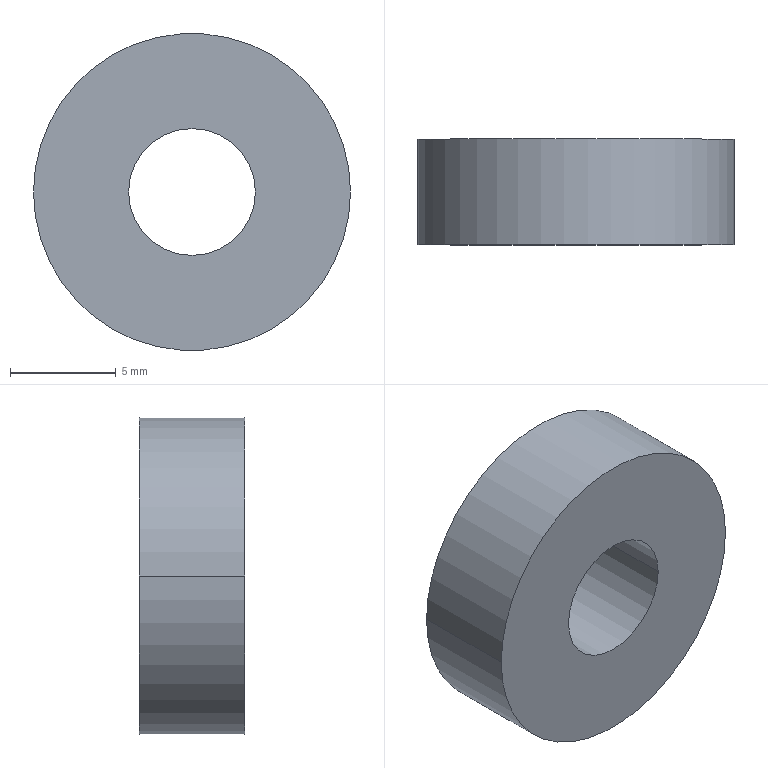Part | SolidWorks | features BaseBody 1 | 1 solid | 6 faces | box 15 x 5 x 15 mm | volume 742.201 mm3 | cylinder 4 | plane 2 | commonest cylinder face diameters 6 x2 15 x2
STEP:
#1=CARTESIAN_POINT('',(3.,5.,0.));
#2=VERTEX_POINT('',#1);
#3=CARTESIAN_POINT('',(-3.,5.,0.));
#4=VERTEX_POINT('',#3);
#5=CARTESIAN_POINT('',(0.,5.,0.));
#6=DIRECTION('',(0.,1.,0.));
#7=DIRECTION('',(1.,0.,0.));
#8=AXIS2_PLACEMENT_3D('',#5,#6,#7);
#9=CIRCLE('',#8,3.);
#10=EDGE_CURVE('',#2,#4,#9,.T.);
#11=ORIENTED_EDGE('',*,*,#10,.T.);
#12=CARTESIAN_POINT('',(-3.,0.,0.));
#13=VERTEX_POINT('',#12);
#14=CARTESIAN_POINT('',(-3.,5.,0.));
#15=DIRECTION('',(0.,-1.,0.));
#16=VECTOR('',#15,1000.);
#17=LINE('',#14,#16);
#18=EDGE_CURVE('',#4,#13,#17,.T.);
#19=ORIENTED_EDGE('',*,*,#18,.T.);
#20=CARTESIAN_POINT('',(3.,0.,0.));
#21=VERTEX_POINT('',#20);
#22=CARTESIAN_POINT('',(0.,0.,0.));
#23=DIRECTION('',(0.,-1.,0.));
#24=DIRECTION('',(1.,0.,0.));
#25=AXIS2_PLACEMENT_3D('',#22,#23,#24);
#26=CIRCLE('',#25,3.);
#27=EDGE_CURVE('',#13,#21,#26,.T.);
#28=ORIENTED_EDGE('',*,*,#27,.T.);
#29=CARTESIAN_POINT('',(3.,5.,0.));
#30=DIRECTION('',(0.,-1.,0.));
#31=VECTOR('',#30,1000.);
#32=LINE('',#29,#31);
#33=EDGE_CURVE('',#2,#21,#32,.T.);
#34=ORIENTED_EDGE('',*,*,#33,.F.);
#35=EDGE_LOOP('',(#11,#19,#28,#34));
#36=FACE_OUTER_BOUND('',#35,.T.);
#37=CARTESIAN_POINT('',(0.,5.,0.));
#38=DIRECTION('',(0.,-1.,0.));
#39=DIRECTION('',(1.,0.,0.));
#40=AXIS2_PLACEMENT_3D('',#37,#38,#39);
#41=CYLINDRICAL_SURFACE('',#40,3.);
#42=ADVANCED_FACE('',(#36),#41,.F.);
#43=CARTESIAN_POINT('',(-7.5,5.,0.));
#44=VERTEX_POINT('',#43);
#45=CARTESIAN_POINT('',(7.5,5.,0.));
#46=VERTEX_POINT('',#45);
#47=CARTESIAN_POINT('',(0.,5.,0.));
#48=DIRECTION('',(0.,1.,0.));
#49=DIRECTION('',(1.,0.,0.));
#50=AXIS2_PLACEMENT_3D('',#47,#48,#49);
#51=CIRCLE('',#50,7.5);
#52=EDGE_CURVE('',#44,#46,#51,.T.);
#53=ORIENTED_EDGE('',*,*,#52,.F.);
#54=CARTESIAN_POINT('',(-7.5,0.,0.));
#55=VERTEX_POINT('',#54);
#56=CARTESIAN_POINT('',(-7.5,5.,0.));
#57=DIRECTION('',(0.,-1.,0.));
#58=VECTOR('',#57,1000.);
#59=LINE('',#56,#58);
#60=EDGE_CURVE('',#44,#55,#59,.T.);
#61=ORIENTED_EDGE('',*,*,#60,.T.);
#62=CARTESIAN_POINT('',(7.5,0.,0.));
#63=VERTEX_POINT('',#62);
#64=CARTESIAN_POINT('',(0.,0.,0.));
#65=DIRECTION('',(0.,1.,0.));
#66=DIRECTION('',(1.,0.,0.));
#67=AXIS2_PLACEMENT_3D('',#64,#65,#66);
#68=CIRCLE('',#67,7.5);
#69=EDGE_CURVE('',#55,#63,#68,.T.);
#70=ORIENTED_EDGE('',*,*,#69,.T.);
#71=CARTESIAN_POINT('',(7.5,5.,0.));
#72=DIRECTION('',(0.,-1.,0.));
#73=VECTOR('',#72,1000.);
#74=LINE('',#71,#73);
#75=EDGE_CURVE('',#46,#63,#74,.T.);
#76=ORIENTED_EDGE('',*,*,#75,.F.);
#77=EDGE_LOOP('',(#53,#61,#70,#76));
#78=FACE_OUTER_BOUND('',#77,.T.);
#79=CARTESIAN_POINT('',(0.,5.,0.));
#80=DIRECTION('',(0.,-1.,0.));
#81=DIRECTION('',(1.,0.,0.));
#82=AXIS2_PLACEMENT_3D('',#79,#80,#81);
#83=CYLINDRICAL_SURFACE('',#82,7.5);
#84=ADVANCED_FACE('',(#78),#83,.T.);
#85=ORIENTED_EDGE('',*,*,#18,.F.);
#86=CARTESIAN_POINT('',(0.,5.,0.));
#87=DIRECTION('',(0.,1.,0.));
#88=DIRECTION('',(1.,0.,0.));
#89=AXIS2_PLACEMENT_3D('',#86,#87,#88);
#90=CIRCLE('',#89,3.);
#91=EDGE_CURVE('',#4,#2,#90,.T.);
#92=ORIENTED_EDGE('',*,*,#91,.T.);
#93=ORIENTED_EDGE('',*,*,#33,.T.);
#94=CARTESIAN_POINT('',(0.,0.,0.));
#95=DIRECTION('',(0.,-1.,0.));
#96=DIRECTION('',(1.,0.,0.));
#97=AXIS2_PLACEMENT_3D('',#94,#95,#96);
#98=CIRCLE('',#97,3.);
#99=EDGE_CURVE('',#21,#13,#98,.T.);
#100=ORIENTED_EDGE('',*,*,#99,.T.);
#101=EDGE_LOOP('',(#85,#92,#93,#100));
#102=FACE_OUTER_BOUND('',#101,.T.);
#103=CARTESIAN_POINT('',(0.,5.,0.));
#104=DIRECTION('',(0.,-1.,0.));
#105=DIRECTION('',(1.,0.,0.));
#106=AXIS2_PLACEMENT_3D('',#103,#104,#105);
#107=CYLINDRICAL_SURFACE('',#106,3.);
#108=ADVANCED_FACE('',(#102),#107,.F.);
#109=ORIENTED_EDGE('',*,*,#99,.F.);
#110=ORIENTED_EDGE('',*,*,#27,.F.);
#111=EDGE_LOOP('',(#109,#110));
#112=FACE_BOUND('',#111,.T.);
#113=CARTESIAN_POINT('',(0.,0.,0.));
#114=DIRECTION('',(0.,1.,0.));
#115=DIRECTION('',(1.,0.,0.));
#116=AXIS2_PLACEMENT_3D('',#113,#114,#115);
#117=CIRCLE('',#116,7.5);
#118=EDGE_CURVE('',#63,#55,#117,.T.);
#119=ORIENTED_EDGE('',*,*,#118,.F.);
#120=ORIENTED_EDGE('',*,*,#69,.F.);
#121=EDGE_LOOP('',(#119,#120));
#122=FACE_OUTER_BOUND('',#121,.T.);
#123=CARTESIAN_POINT('',(-7.59,0.,-7.59));
#124=DIRECTION('',(0.,1.,0.));
#125=DIRECTION('',(0.,0.,1.));
#126=AXIS2_PLACEMENT_3D('',#123,#124,#125);
#127=PLANE('',#126);
#128=ADVANCED_FACE('',(#112,#122),#127,.F.);
#129=ORIENTED_EDGE('',*,*,#10,.F.);
#130=ORIENTED_EDGE('',*,*,#91,.F.);
#131=EDGE_LOOP('',(#129,#130));
#132=FACE_BOUND('',#131,.T.);
#133=CARTESIAN_POINT('',(0.,5.,0.));
#134=DIRECTION('',(0.,1.,0.));
#135=DIRECTION('',(1.,0.,0.));
#136=AXIS2_PLACEMENT_3D('',#133,#134,#135);
#137=CIRCLE('',#136,7.5);
#138=EDGE_CURVE('',#46,#44,#137,.T.);
#139=ORIENTED_EDGE('',*,*,#138,.T.);
#140=ORIENTED_EDGE('',*,*,#52,.T.);
#141=EDGE_LOOP('',(#139,#140));
#142=FACE_OUTER_BOUND('',#141,.T.);
#143=CARTESIAN_POINT('',(-7.59,5.,-7.59));
#144=DIRECTION('',(0.,1.,0.));
#145=DIRECTION('',(0.,0.,1.));
#146=AXIS2_PLACEMENT_3D('',#143,#144,#145);
#147=PLANE('',#146);
#148=ADVANCED_FACE('',(#132,#142),#147,.T.);
#149=ORIENTED_EDGE('',*,*,#60,.F.);
#150=ORIENTED_EDGE('',*,*,#138,.F.);
#151=ORIENTED_EDGE('',*,*,#75,.T.);
#152=ORIENTED_EDGE('',*,*,#118,.T.);
#153=EDGE_LOOP('',(#149,#150,#151,#152));
#154=FACE_OUTER_BOUND('',#153,.T.);
#155=CARTESIAN_POINT('',(0.,5.,0.));
#156=DIRECTION('',(0.,-1.,0.));
#157=DIRECTION('',(1.,0.,0.));
#158=AXIS2_PLACEMENT_3D('',#155,#156,#157);
#159=CYLINDRICAL_SURFACE('',#158,7.5);
#160=ADVANCED_FACE('',(#154),#159,.T.);
#161=CLOSED_SHELL('',(#42,#84,#108,#128,#148,#160));
#162=MANIFOLD_SOLID_BREP('',#161);
#163=CARTESIAN_POINT('',(0.,0.,0.));
#164=DIRECTION('',(0.,0.,1.));
#165=DIRECTION('',(1.,0.,0.));
#166=AXIS2_PLACEMENT_3D('',#163,#164,#165);
#167=(LENGTH_UNIT()NAMED_UNIT(*)SI_UNIT(.MILLI.,.METRE.));
#168=UNCERTAINTY_MEASURE_WITH_UNIT(LENGTH_MEASURE(0.00001),#167,'','');
#169=(NAMED_UNIT(*)PLANE_ANGLE_UNIT()SI_UNIT($,.RADIAN.));
#170=(NAMED_UNIT(*)SI_UNIT($,.STERADIAN.)SOLID_ANGLE_UNIT());
#171=(GEOMETRIC_REPRESENTATION_CONTEXT(3)GLOBAL_UNCERTAINTY_ASSIGNED_CONTEXT((#168))GLOBAL_UNIT_ASSIGNED_CONTEXT((#167,#169,#170))REPRESENTATION_CONTEXT('',''));
#172=ADVANCED_BREP_SHAPE_REPRESENTATION('',(#162,#166),#171);